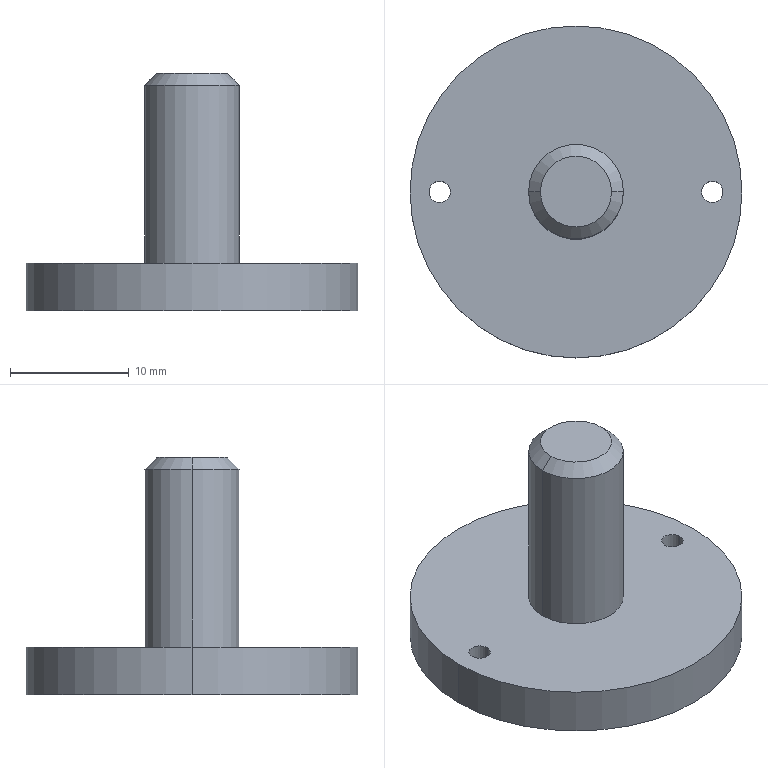Part | STEP file | Clamping screw | 1 solid | 13 faces | box 28 x 28 x 20 mm | volume 3235 mm3 | cylinder 8 | plane 3 | cone 2 | commonest cylinder face diameters 1.8 x4 8 x2 28 x2
STEP:
#1=CARTESIAN_POINT('',(-12.4,0.,4.));
#2=VERTEX_POINT('',#1);
#3=CARTESIAN_POINT('',(-10.6,0.,4.));
#4=VERTEX_POINT('',#3);
#5=CARTESIAN_POINT('',(-11.5,0.,4.));
#6=DIRECTION('',(0.,0.,1.));
#7=DIRECTION('',(1.,0.,0.));
#8=AXIS2_PLACEMENT_3D('',#5,#6,#7);
#9=CIRCLE('',#8,0.9);
#10=EDGE_CURVE('',#2,#4,#9,.T.);
#11=ORIENTED_EDGE('',*,*,#10,.T.);
#12=CARTESIAN_POINT('',(-10.6,0.,0.));
#13=VERTEX_POINT('',#12);
#14=CARTESIAN_POINT('',(-10.6,0.,16.));
#15=DIRECTION('',(0.,0.,-1.));
#16=VECTOR('',#15,1000.);
#17=LINE('',#14,#16);
#18=EDGE_CURVE('',#4,#13,#17,.T.);
#19=ORIENTED_EDGE('',*,*,#18,.T.);
#20=CARTESIAN_POINT('',(-12.4,0.,0.));
#21=VERTEX_POINT('',#20);
#22=CARTESIAN_POINT('',(-11.5,0.,0.));
#23=DIRECTION('',(0.,0.,-1.));
#24=DIRECTION('',(1.,0.,0.));
#25=AXIS2_PLACEMENT_3D('',#22,#23,#24);
#26=CIRCLE('',#25,0.9);
#27=EDGE_CURVE('',#13,#21,#26,.T.);
#28=ORIENTED_EDGE('',*,*,#27,.T.);
#29=CARTESIAN_POINT('',(-12.4,0.,16.));
#30=DIRECTION('',(0.,0.,-1.));
#31=VECTOR('',#30,1000.);
#32=LINE('',#29,#31);
#33=EDGE_CURVE('',#2,#21,#32,.T.);
#34=ORIENTED_EDGE('',*,*,#33,.F.);
#35=EDGE_LOOP('',(#11,#19,#28,#34));
#36=FACE_OUTER_BOUND('',#35,.T.);
#37=CARTESIAN_POINT('',(-11.5,0.,16.));
#38=DIRECTION('',(0.,0.,-1.));
#39=DIRECTION('',(-1.,0.,0.));
#40=AXIS2_PLACEMENT_3D('',#37,#38,#39);
#41=CYLINDRICAL_SURFACE('',#40,0.9);
#42=ADVANCED_FACE('',(#36),#41,.F.);
#43=CARTESIAN_POINT('',(10.6,0.,4.));
#44=VERTEX_POINT('',#43);
#45=CARTESIAN_POINT('',(12.4,0.,4.));
#46=VERTEX_POINT('',#45);
#47=CARTESIAN_POINT('',(11.5,0.,4.));
#48=DIRECTION('',(0.,0.,1.));
#49=DIRECTION('',(1.,0.,0.));
#50=AXIS2_PLACEMENT_3D('',#47,#48,#49);
#51=CIRCLE('',#50,0.9);
#52=EDGE_CURVE('',#44,#46,#51,.T.);
#53=ORIENTED_EDGE('',*,*,#52,.T.);
#54=CARTESIAN_POINT('',(12.4,0.,0.));
#55=VERTEX_POINT('',#54);
#56=CARTESIAN_POINT('',(12.4,0.,16.));
#57=DIRECTION('',(0.,0.,-1.));
#58=VECTOR('',#57,1000.);
#59=LINE('',#56,#58);
#60=EDGE_CURVE('',#46,#55,#59,.T.);
#61=ORIENTED_EDGE('',*,*,#60,.T.);
#62=CARTESIAN_POINT('',(10.6,0.,0.));
#63=VERTEX_POINT('',#62);
#64=CARTESIAN_POINT('',(11.5,0.,0.));
#65=DIRECTION('',(0.,0.,-1.));
#66=DIRECTION('',(-1.,0.,0.));
#67=AXIS2_PLACEMENT_3D('',#64,#65,#66);
#68=CIRCLE('',#67,0.9);
#69=EDGE_CURVE('',#55,#63,#68,.T.);
#70=ORIENTED_EDGE('',*,*,#69,.T.);
#71=CARTESIAN_POINT('',(10.6,0.,16.));
#72=DIRECTION('',(0.,0.,-1.));
#73=VECTOR('',#72,1000.);
#74=LINE('',#71,#73);
#75=EDGE_CURVE('',#44,#63,#74,.T.);
#76=ORIENTED_EDGE('',*,*,#75,.F.);
#77=EDGE_LOOP('',(#53,#61,#70,#76));
#78=FACE_OUTER_BOUND('',#77,.T.);
#79=CARTESIAN_POINT('',(11.5,0.,16.));
#80=DIRECTION('',(0.,0.,-1.));
#81=DIRECTION('',(-1.,0.,0.));
#82=AXIS2_PLACEMENT_3D('',#79,#80,#81);
#83=CYLINDRICAL_SURFACE('',#82,0.9);
#84=ADVANCED_FACE('',(#78),#83,.F.);
#85=CARTESIAN_POINT('',(3.,0.,20.));
#86=VERTEX_POINT('',#85);
#87=CARTESIAN_POINT('',(-3.,0.,20.));
#88=VERTEX_POINT('',#87);
#89=CARTESIAN_POINT('',(0.,0.,20.));
#90=DIRECTION('',(0.,0.,1.));
#91=DIRECTION('',(1.,0.,0.));
#92=AXIS2_PLACEMENT_3D('',#89,#90,#91);
#93=CIRCLE('',#92,3.);
#94=EDGE_CURVE('',#86,#88,#93,.T.);
#95=ORIENTED_EDGE('',*,*,#94,.F.);
#96=CARTESIAN_POINT('',(4.,0.,19.));
#97=VERTEX_POINT('',#96);
#98=CARTESIAN_POINT('',(3.,0.,20.));
#99=DIRECTION('',(0.7071,0.,-0.7071));
#100=VECTOR('',#99,1000.);
#101=LINE('',#98,#100);
#102=EDGE_CURVE('',#86,#97,#101,.T.);
#103=ORIENTED_EDGE('',*,*,#102,.T.);
#104=CARTESIAN_POINT('',(-4.,0.,19.));
#105=VERTEX_POINT('',#104);
#106=CARTESIAN_POINT('',(0.,0.,19.));
#107=DIRECTION('',(0.,0.,-1.));
#108=DIRECTION('',(1.,0.,0.));
#109=AXIS2_PLACEMENT_3D('',#106,#107,#108);
#110=CIRCLE('',#109,4.);
#111=EDGE_CURVE('',#105,#97,#110,.T.);
#112=ORIENTED_EDGE('',*,*,#111,.F.);
#113=CARTESIAN_POINT('',(-3.,0.,20.));
#114=DIRECTION('',(-0.7071,0.,-0.7071));
#115=VECTOR('',#114,1000.);
#116=LINE('',#113,#115);
#117=EDGE_CURVE('',#88,#105,#116,.T.);
#118=ORIENTED_EDGE('',*,*,#117,.F.);
#119=EDGE_LOOP('',(#95,#103,#112,#118));
#120=FACE_OUTER_BOUND('',#119,.T.);
#121=CARTESIAN_POINT('',(0.,0.,20.));
#122=DIRECTION('',(0.,0.,-1.));
#123=DIRECTION('',(-1.,0.,0.));
#124=AXIS2_PLACEMENT_3D('',#121,#122,#123);
#125=CONICAL_SURFACE('',#124,3.,0.7854);
#126=ADVANCED_FACE('',(#120),#125,.T.);
#127=ORIENTED_EDGE('',*,*,#111,.T.);
#128=CARTESIAN_POINT('',(4.,0.,4.));
#129=VERTEX_POINT('',#128);
#130=CARTESIAN_POINT('',(4.,0.,20.));
#131=DIRECTION('',(0.,0.,-1.));
#132=VECTOR('',#131,1000.);
#133=LINE('',#130,#132);
#134=EDGE_CURVE('',#97,#129,#133,.T.);
#135=ORIENTED_EDGE('',*,*,#134,.T.);
#136=CARTESIAN_POINT('',(-4.,0.,4.));
#137=VERTEX_POINT('',#136);
#138=CARTESIAN_POINT('',(0.,0.,4.));
#139=DIRECTION('',(0.,0.,1.));
#140=DIRECTION('',(1.,0.,0.));
#141=AXIS2_PLACEMENT_3D('',#138,#139,#140);
#142=CIRCLE('',#141,4.);
#143=EDGE_CURVE('',#129,#137,#142,.T.);
#144=ORIENTED_EDGE('',*,*,#143,.T.);
#145=CARTESIAN_POINT('',(-4.,0.,20.));
#146=DIRECTION('',(0.,0.,-1.));
#147=VECTOR('',#146,1000.);
#148=LINE('',#145,#147);
#149=EDGE_CURVE('',#105,#137,#148,.T.);
#150=ORIENTED_EDGE('',*,*,#149,.F.);
#151=EDGE_LOOP('',(#127,#135,#144,#150));
#152=FACE_OUTER_BOUND('',#151,.T.);
#153=CARTESIAN_POINT('',(0.,0.,20.));
#154=DIRECTION('',(0.,0.,-1.));
#155=DIRECTION('',(-1.,0.,0.));
#156=AXIS2_PLACEMENT_3D('',#153,#154,#155);
#157=CYLINDRICAL_SURFACE('',#156,4.);
#158=ADVANCED_FACE('',(#152),#157,.T.);
#159=CARTESIAN_POINT('',(14.,0.,4.));
#160=VERTEX_POINT('',#159);
#161=CARTESIAN_POINT('',(-14.,0.,4.));
#162=VERTEX_POINT('',#161);
#163=CARTESIAN_POINT('',(0.,0.,4.));
#164=DIRECTION('',(0.,0.,1.));
#165=DIRECTION('',(1.,0.,0.));
#166=AXIS2_PLACEMENT_3D('',#163,#164,#165);
#167=CIRCLE('',#166,14.);
#168=EDGE_CURVE('',#160,#162,#167,.T.);
#169=ORIENTED_EDGE('',*,*,#168,.F.);
#170=CARTESIAN_POINT('',(14.,0.,0.));
#171=VERTEX_POINT('',#170);
#172=CARTESIAN_POINT('',(14.,0.,4.));
#173=DIRECTION('',(0.,0.,-1.));
#174=VECTOR('',#173,1000.);
#175=LINE('',#172,#174);
#176=EDGE_CURVE('',#160,#171,#175,.T.);
#177=ORIENTED_EDGE('',*,*,#176,.T.);
#178=CARTESIAN_POINT('',(-14.,0.,0.));
#179=VERTEX_POINT('',#178);
#180=CARTESIAN_POINT('',(0.,0.,0.));
#181=DIRECTION('',(0.,0.,1.));
#182=DIRECTION('',(1.,0.,0.));
#183=AXIS2_PLACEMENT_3D('',#180,#181,#182);
#184=CIRCLE('',#183,14.);
#185=EDGE_CURVE('',#171,#179,#184,.T.);
#186=ORIENTED_EDGE('',*,*,#185,.T.);
#187=CARTESIAN_POINT('',(-14.,0.,4.));
#188=DIRECTION('',(0.,0.,-1.));
#189=VECTOR('',#188,1000.);
#190=LINE('',#187,#189);
#191=EDGE_CURVE('',#162,#179,#190,.T.);
#192=ORIENTED_EDGE('',*,*,#191,.F.);
#193=EDGE_LOOP('',(#169,#177,#186,#192));
#194=FACE_OUTER_BOUND('',#193,.T.);
#195=CARTESIAN_POINT('',(0.,0.,4.));
#196=DIRECTION('',(0.,0.,-1.));
#197=DIRECTION('',(-1.,0.,0.));
#198=AXIS2_PLACEMENT_3D('',#195,#196,#197);
#199=CYLINDRICAL_SURFACE('',#198,14.);
#200=ADVANCED_FACE('',(#194),#199,.T.);
#201=ORIENTED_EDGE('',*,*,#176,.F.);
#202=CARTESIAN_POINT('',(0.,0.,4.));
#203=DIRECTION('',(0.,0.,1.));
#204=DIRECTION('',(1.,0.,0.));
#205=AXIS2_PLACEMENT_3D('',#202,#203,#204);
#206=CIRCLE('',#205,14.);
#207=EDGE_CURVE('',#162,#160,#206,.T.);
#208=ORIENTED_EDGE('',*,*,#207,.F.);
#209=ORIENTED_EDGE('',*,*,#191,.T.);
#210=CARTESIAN_POINT('',(0.,0.,0.));
#211=DIRECTION('',(0.,0.,1.));
#212=DIRECTION('',(1.,0.,0.));
#213=AXIS2_PLACEMENT_3D('',#210,#211,#212);
#214=CIRCLE('',#213,14.);
#215=EDGE_CURVE('',#179,#171,#214,.T.);
#216=ORIENTED_EDGE('',*,*,#215,.T.);
#217=EDGE_LOOP('',(#201,#208,#209,#216));
#218=FACE_OUTER_BOUND('',#217,.T.);
#219=CARTESIAN_POINT('',(0.,0.,4.));
#220=DIRECTION('',(0.,0.,-1.));
#221=DIRECTION('',(-1.,0.,0.));
#222=AXIS2_PLACEMENT_3D('',#219,#220,#221);
#223=CYLINDRICAL_SURFACE('',#222,14.);
#224=ADVANCED_FACE('',(#218),#223,.T.);
#225=ORIENTED_EDGE('',*,*,#10,.F.);
#226=CARTESIAN_POINT('',(-11.5,0.,4.));
#227=DIRECTION('',(0.,0.,1.));
#228=DIRECTION('',(1.,0.,0.));
#229=AXIS2_PLACEMENT_3D('',#226,#227,#228);
#230=CIRCLE('',#229,0.9);
#231=EDGE_CURVE('',#4,#2,#230,.T.);
#232=ORIENTED_EDGE('',*,*,#231,.F.);
#233=EDGE_LOOP('',(#225,#232));
#234=FACE_BOUND('',#233,.T.);
#235=ORIENTED_EDGE('',*,*,#52,.F.);
#236=CARTESIAN_POINT('',(11.5,0.,4.));
#237=DIRECTION('',(0.,0.,1.));
#238=DIRECTION('',(1.,0.,0.));
#239=AXIS2_PLACEMENT_3D('',#236,#237,#238);
#240=CIRCLE('',#239,0.9);
#241=EDGE_CURVE('',#46,#44,#240,.T.);
#242=ORIENTED_EDGE('',*,*,#241,.F.);
#243=EDGE_LOOP('',(#235,#242));
#244=FACE_BOUND('',#243,.T.);
#245=CARTESIAN_POINT('',(0.,0.,4.));
#246=DIRECTION('',(0.,0.,1.));
#247=DIRECTION('',(1.,0.,0.));
#248=AXIS2_PLACEMENT_3D('',#245,#246,#247);
#249=CIRCLE('',#248,4.);
#250=EDGE_CURVE('',#137,#129,#249,.T.);
#251=ORIENTED_EDGE('',*,*,#250,.F.);
#252=ORIENTED_EDGE('',*,*,#143,.F.);
#253=EDGE_LOOP('',(#251,#252));
#254=FACE_BOUND('',#253,.T.);
#255=ORIENTED_EDGE('',*,*,#207,.T.);
#256=ORIENTED_EDGE('',*,*,#168,.T.);
#257=EDGE_LOOP('',(#255,#256));
#258=FACE_OUTER_BOUND('',#257,.T.);
#259=CARTESIAN_POINT('',(0.,0.,4.));
#260=DIRECTION('',(0.,0.,1.));
#261=DIRECTION('',(1.,0.,0.));
#262=AXIS2_PLACEMENT_3D('',#259,#260,#261);
#263=PLANE('',#262);
#264=ADVANCED_FACE('',(#234,#244,#254,#258),#263,.T.);
#265=CARTESIAN_POINT('',(-11.5,0.,0.));
#266=DIRECTION('',(0.,0.,-1.));
#267=DIRECTION('',(1.,0.,0.));
#268=AXIS2_PLACEMENT_3D('',#265,#266,#267);
#269=CIRCLE('',#268,0.9);
#270=EDGE_CURVE('',#21,#13,#269,.T.);
#271=ORIENTED_EDGE('',*,*,#270,.F.);
#272=ORIENTED_EDGE('',*,*,#27,.F.);
#273=EDGE_LOOP('',(#271,#272));
#274=FACE_BOUND('',#273,.T.);
#275=CARTESIAN_POINT('',(11.5,0.,0.));
#276=DIRECTION('',(0.,0.,-1.));
#277=DIRECTION('',(-1.,0.,0.));
#278=AXIS2_PLACEMENT_3D('',#275,#276,#277);
#279=CIRCLE('',#278,0.9);
#280=EDGE_CURVE('',#63,#55,#279,.T.);
#281=ORIENTED_EDGE('',*,*,#280,.F.);
#282=ORIENTED_EDGE('',*,*,#69,.F.);
#283=EDGE_LOOP('',(#281,#282));
#284=FACE_BOUND('',#283,.T.);
#285=ORIENTED_EDGE('',*,*,#215,.F.);
#286=ORIENTED_EDGE('',*,*,#185,.F.);
#287=EDGE_LOOP('',(#285,#286));
#288=FACE_OUTER_BOUND('',#287,.T.);
#289=CARTESIAN_POINT('',(0.,0.,0.));
#290=DIRECTION('',(0.,0.,1.));
#291=DIRECTION('',(1.,0.,0.));
#292=AXIS2_PLACEMENT_3D('',#289,#290,#291);
#293=PLANE('',#292);
#294=ADVANCED_FACE('',(#274,#284,#288),#293,.F.);
#295=ORIENTED_EDGE('',*,*,#134,.F.);
#296=CARTESIAN_POINT('',(0.,0.,19.));
#297=DIRECTION('',(0.,0.,-1.));
#298=DIRECTION('',(1.,0.,0.));
#299=AXIS2_PLACEMENT_3D('',#296,#297,#298);
#300=CIRCLE('',#299,4.);
#301=EDGE_CURVE('',#97,#105,#300,.T.);
#302=ORIENTED_EDGE('',*,*,#301,.T.);
#303=ORIENTED_EDGE('',*,*,#149,.T.);
#304=ORIENTED_EDGE('',*,*,#250,.T.);
#305=EDGE_LOOP('',(#295,#302,#303,#304));
#306=FACE_OUTER_BOUND('',#305,.T.);
#307=CARTESIAN_POINT('',(0.,0.,20.));
#308=DIRECTION('',(0.,0.,-1.));
#309=DIRECTION('',(-1.,0.,0.));
#310=AXIS2_PLACEMENT_3D('',#307,#308,#309);
#311=CYLINDRICAL_SURFACE('',#310,4.);
#312=ADVANCED_FACE('',(#306),#311,.T.);
#313=CARTESIAN_POINT('',(0.,0.,20.));
#314=DIRECTION('',(0.,0.,1.));
#315=DIRECTION('',(1.,0.,0.));
#316=AXIS2_PLACEMENT_3D('',#313,#314,#315);
#317=CIRCLE('',#316,3.);
#318=EDGE_CURVE('',#88,#86,#317,.T.);
#319=ORIENTED_EDGE('',*,*,#318,.T.);
#320=ORIENTED_EDGE('',*,*,#94,.T.);
#321=EDGE_LOOP('',(#319,#320));
#322=FACE_OUTER_BOUND('',#321,.T.);
#323=CARTESIAN_POINT('',(0.,0.,20.));
#324=DIRECTION('',(0.,0.,1.));
#325=DIRECTION('',(1.,0.,0.));
#326=AXIS2_PLACEMENT_3D('',#323,#324,#325);
#327=PLANE('',#326);
#328=ADVANCED_FACE('',(#322),#327,.T.);
#329=ORIENTED_EDGE('',*,*,#102,.F.);
#330=ORIENTED_EDGE('',*,*,#318,.F.);
#331=ORIENTED_EDGE('',*,*,#117,.T.);
#332=ORIENTED_EDGE('',*,*,#301,.F.);
#333=EDGE_LOOP('',(#329,#330,#331,#332));
#334=FACE_OUTER_BOUND('',#333,.T.);
#335=CARTESIAN_POINT('',(0.,0.,20.));
#336=DIRECTION('',(0.,0.,-1.));
#337=DIRECTION('',(-1.,0.,0.));
#338=AXIS2_PLACEMENT_3D('',#335,#336,#337);
#339=CONICAL_SURFACE('',#338,3.,0.7854);
#340=ADVANCED_FACE('',(#334),#339,.T.);
#341=ORIENTED_EDGE('',*,*,#60,.F.);
#342=ORIENTED_EDGE('',*,*,#241,.T.);
#343=ORIENTED_EDGE('',*,*,#75,.T.);
#344=ORIENTED_EDGE('',*,*,#280,.T.);
#345=EDGE_LOOP('',(#341,#342,#343,#344));
#346=FACE_OUTER_BOUND('',#345,.T.);
#347=CARTESIAN_POINT('',(11.5,0.,16.));
#348=DIRECTION('',(0.,0.,-1.));
#349=DIRECTION('',(-1.,0.,0.));
#350=AXIS2_PLACEMENT_3D('',#347,#348,#349);
#351=CYLINDRICAL_SURFACE('',#350,0.9);
#352=ADVANCED_FACE('',(#346),#351,.F.);
#353=ORIENTED_EDGE('',*,*,#18,.F.);
#354=ORIENTED_EDGE('',*,*,#231,.T.);
#355=ORIENTED_EDGE('',*,*,#33,.T.);
#356=ORIENTED_EDGE('',*,*,#270,.T.);
#357=EDGE_LOOP('',(#353,#354,#355,#356));
#358=FACE_OUTER_BOUND('',#357,.T.);
#359=CARTESIAN_POINT('',(-11.5,0.,16.));
#360=DIRECTION('',(0.,0.,-1.));
#361=DIRECTION('',(-1.,0.,0.));
#362=AXIS2_PLACEMENT_3D('',#359,#360,#361);
#363=CYLINDRICAL_SURFACE('',#362,0.9);
#364=ADVANCED_FACE('',(#358),#363,.F.);
#365=CLOSED_SHELL('',(#42,#84,#126,#158,#200,#224,#264,#294,#312,#328,#340,#352,#364));
#366=MANIFOLD_SOLID_BREP('',#365);
#367=CARTESIAN_POINT('',(0.,0.,0.));
#368=DIRECTION('',(0.,0.,1.));
#369=DIRECTION('',(1.,0.,0.));
#370=AXIS2_PLACEMENT_3D('',#367,#368,#369);
#371=(LENGTH_UNIT()NAMED_UNIT(*)SI_UNIT(.MILLI.,.METRE.));
#372=UNCERTAINTY_MEASURE_WITH_UNIT(LENGTH_MEASURE(0.00001),#371,'','');
#373=(NAMED_UNIT(*)PLANE_ANGLE_UNIT()SI_UNIT($,.RADIAN.));
#374=(NAMED_UNIT(*)SI_UNIT($,.STERADIAN.)SOLID_ANGLE_UNIT());
#375=(GEOMETRIC_REPRESENTATION_CONTEXT(3)GLOBAL_UNCERTAINTY_ASSIGNED_CONTEXT((#372))GLOBAL_UNIT_ASSIGNED_CONTEXT((#371,#373,#374))REPRESENTATION_CONTEXT('',''));
#376=ADVANCED_BREP_SHAPE_REPRESENTATION('',(#366,#370),#375);